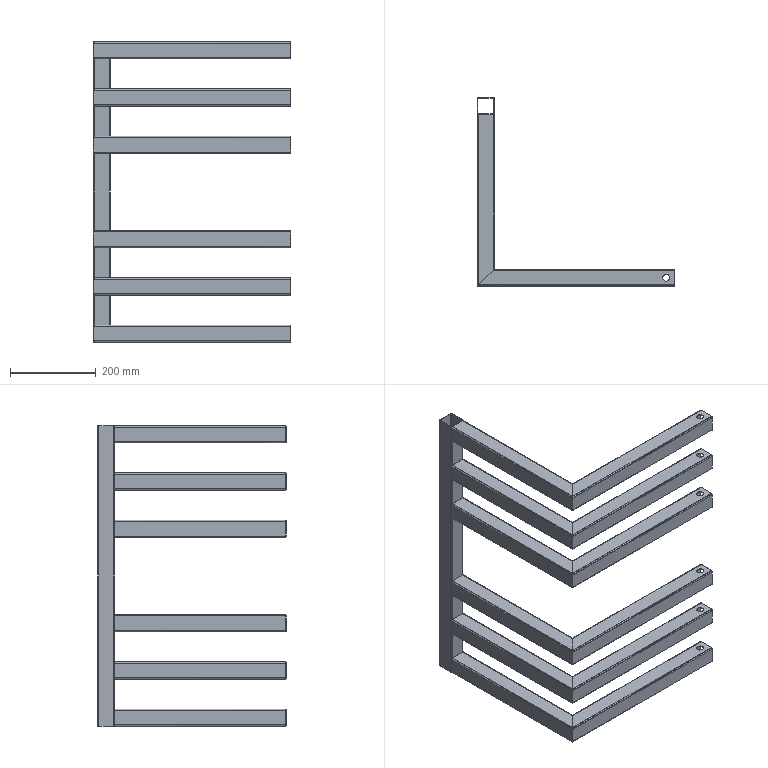Part | SolidWorks | features 3DProfileFeature 1, ICE 1, LPattern 1, WeldMemberFeat 1, WeldmentFeature 1 | 13 solids | 258 faces | box 460 x 440 x 700 mm | volume 1262037 mm3 | plane 130 | cylinder 128 | commonest cylinder face diameters 3 x52 6 x52 16 x24